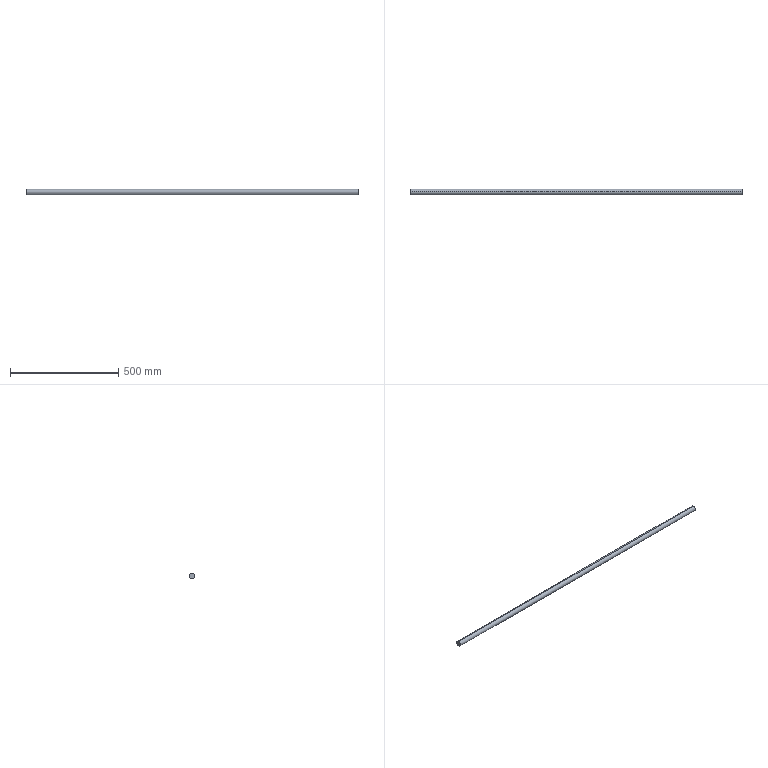Part | SolidWorks | features ICE 1, MirrorPattern 1, Revolution 1 | 1 solid | 4 faces | box 1534 x 25 x 25 mm | volume 753000 mm3 | cylinder 2 | plane 2 | commonest cylinder face diameters 25 x2
STEP:
#1=CARTESIAN_POINT('',(767.,0.,12.5));
#2=VERTEX_POINT('',#1);
#3=CARTESIAN_POINT('',(767.,0.,-12.5));
#4=VERTEX_POINT('',#3);
#5=CARTESIAN_POINT('',(767.,0.,0.));
#6=DIRECTION('',(-1.,0.,0.));
#7=DIRECTION('',(0.,0.,1.));
#8=AXIS2_PLACEMENT_3D('',#5,#6,#7);
#9=CIRCLE('',#8,12.5);
#10=EDGE_CURVE('',#2,#4,#9,.T.);
#11=ORIENTED_EDGE('',*,*,#10,.T.);
#12=CARTESIAN_POINT('',(-767.,0.,-12.5));
#13=VERTEX_POINT('',#12);
#14=CARTESIAN_POINT('',(-202.604,0.,-12.5));
#15=DIRECTION('',(-1.,0.,0.));
#16=VECTOR('',#15,1000.);
#17=LINE('',#14,#16);
#18=EDGE_CURVE('',#4,#13,#17,.T.);
#19=ORIENTED_EDGE('',*,*,#18,.T.);
#20=CARTESIAN_POINT('',(-767.,0.,12.5));
#21=VERTEX_POINT('',#20);
#22=CARTESIAN_POINT('',(-767.,0.,0.));
#23=DIRECTION('',(-1.,0.,0.));
#24=DIRECTION('',(0.,0.,1.));
#25=AXIS2_PLACEMENT_3D('',#22,#23,#24);
#26=CIRCLE('',#25,12.5);
#27=EDGE_CURVE('',#21,#13,#26,.T.);
#28=ORIENTED_EDGE('',*,*,#27,.F.);
#29=CARTESIAN_POINT('',(-202.604,0.,12.5));
#30=DIRECTION('',(-1.,0.,0.));
#31=VECTOR('',#30,1000.);
#32=LINE('',#29,#31);
#33=EDGE_CURVE('',#2,#21,#32,.T.);
#34=ORIENTED_EDGE('',*,*,#33,.F.);
#35=EDGE_LOOP('',(#11,#19,#28,#34));
#36=FACE_OUTER_BOUND('',#35,.T.);
#37=CARTESIAN_POINT('',(-202.604,0.,0.));
#38=DIRECTION('',(-1.,0.,0.));
#39=DIRECTION('',(0.,0.,1.));
#40=AXIS2_PLACEMENT_3D('',#37,#38,#39);
#41=CYLINDRICAL_SURFACE('',#40,12.5);
#42=ADVANCED_FACE('',(#36),#41,.T.);
#43=ORIENTED_EDGE('',*,*,#27,.T.);
#44=CARTESIAN_POINT('',(-767.,0.,0.));
#45=DIRECTION('',(-1.,0.,0.));
#46=DIRECTION('',(0.,0.,1.));
#47=AXIS2_PLACEMENT_3D('',#44,#45,#46);
#48=CIRCLE('',#47,12.5);
#49=EDGE_CURVE('',#13,#21,#48,.T.);
#50=ORIENTED_EDGE('',*,*,#49,.T.);
#51=EDGE_LOOP('',(#43,#50));
#52=FACE_OUTER_BOUND('',#51,.T.);
#53=CARTESIAN_POINT('',(-767.,0.,0.));
#54=DIRECTION('',(1.,0.,0.));
#55=DIRECTION('',(0.,0.,-1.));
#56=AXIS2_PLACEMENT_3D('',#53,#54,#55);
#57=PLANE('',#56);
#58=ADVANCED_FACE('',(#52),#57,.F.);
#59=ORIENTED_EDGE('',*,*,#18,.F.);
#60=CARTESIAN_POINT('',(767.,0.,0.));
#61=DIRECTION('',(-1.,0.,0.));
#62=DIRECTION('',(0.,0.,1.));
#63=AXIS2_PLACEMENT_3D('',#60,#61,#62);
#64=CIRCLE('',#63,12.5);
#65=EDGE_CURVE('',#4,#2,#64,.T.);
#66=ORIENTED_EDGE('',*,*,#65,.T.);
#67=ORIENTED_EDGE('',*,*,#33,.T.);
#68=ORIENTED_EDGE('',*,*,#49,.F.);
#69=EDGE_LOOP('',(#59,#66,#67,#68));
#70=FACE_OUTER_BOUND('',#69,.T.);
#71=CARTESIAN_POINT('',(-202.604,0.,0.));
#72=DIRECTION('',(-1.,0.,0.));
#73=DIRECTION('',(0.,0.,1.));
#74=AXIS2_PLACEMENT_3D('',#71,#72,#73);
#75=CYLINDRICAL_SURFACE('',#74,12.5);
#76=ADVANCED_FACE('',(#70),#75,.T.);
#77=ORIENTED_EDGE('',*,*,#10,.F.);
#78=ORIENTED_EDGE('',*,*,#65,.F.);
#79=EDGE_LOOP('',(#77,#78));
#80=FACE_OUTER_BOUND('',#79,.T.);
#81=CARTESIAN_POINT('',(767.,0.,0.));
#82=DIRECTION('',(-1.,0.,0.));
#83=DIRECTION('',(0.,0.,-1.));
#84=AXIS2_PLACEMENT_3D('',#81,#82,#83);
#85=PLANE('',#84);
#86=ADVANCED_FACE('',(#80),#85,.F.);
#87=CLOSED_SHELL('',(#42,#58,#76,#86));
#88=MANIFOLD_SOLID_BREP('',#87);
#89=CARTESIAN_POINT('',(0.,0.,0.));
#90=DIRECTION('',(0.,0.,1.));
#91=DIRECTION('',(1.,0.,0.));
#92=AXIS2_PLACEMENT_3D('',#89,#90,#91);
#93=(LENGTH_UNIT()NAMED_UNIT(*)SI_UNIT(.MILLI.,.METRE.));
#94=UNCERTAINTY_MEASURE_WITH_UNIT(LENGTH_MEASURE(0.00001),#93,'','');
#95=(NAMED_UNIT(*)PLANE_ANGLE_UNIT()SI_UNIT($,.RADIAN.));
#96=(NAMED_UNIT(*)SI_UNIT($,.STERADIAN.)SOLID_ANGLE_UNIT());
#97=(GEOMETRIC_REPRESENTATION_CONTEXT(3)GLOBAL_UNCERTAINTY_ASSIGNED_CONTEXT((#94))GLOBAL_UNIT_ASSIGNED_CONTEXT((#93,#95,#96))REPRESENTATION_CONTEXT('',''));
#98=ADVANCED_BREP_SHAPE_REPRESENTATION('',(#88,#92),#97);